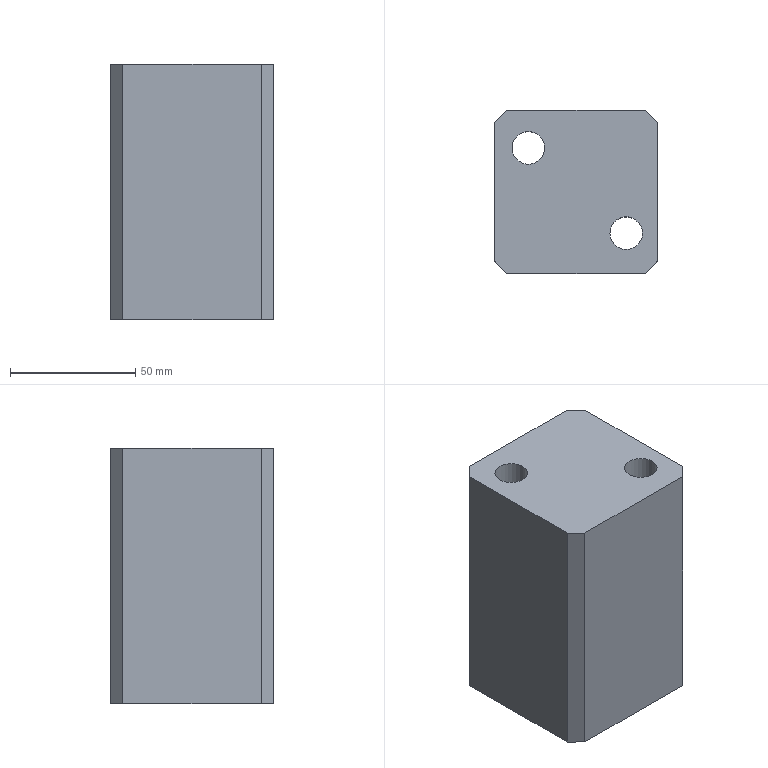Part | STEP file | 218-1_id198_x_t | 1 solid | 22 faces | box 65 x 65 x 102 mm | volume 370243 mm3 | plane 12 | cylinder 6 | cone 4 | commonest cylinder face diameters 10.3 x2 13 x2 20 x2